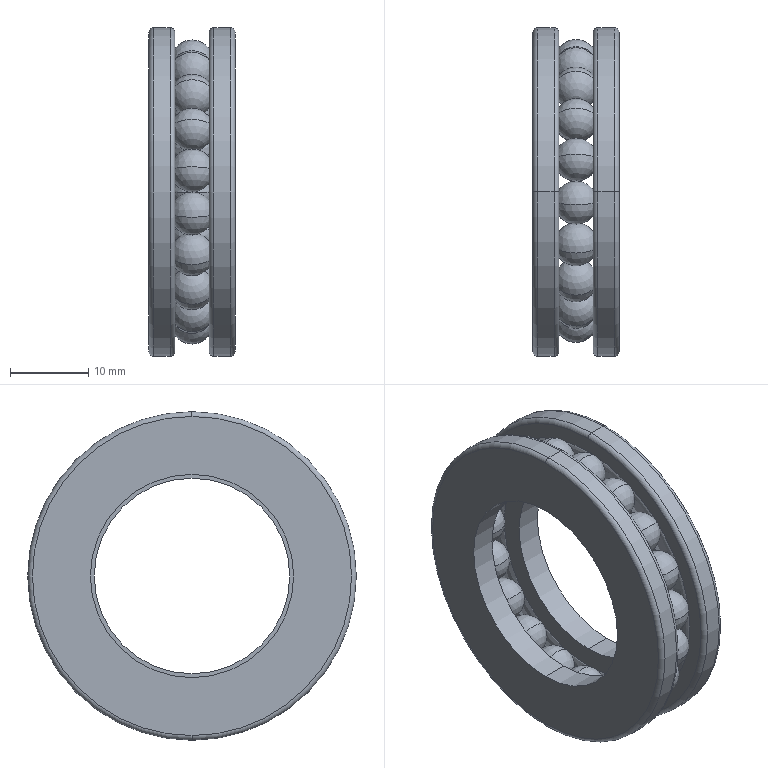Part | SolidWorks | features Revolution 3, CirPattern 1, Fillet 1 | 1 solid | 100 faces | box 11 x 42 x 42 mm | volume 7140 mm3 | torus 48 | sphere 38 | cylinder 8 | plane 6 | commonest cylinder face diameters 42 x4 25 x2 26 x2